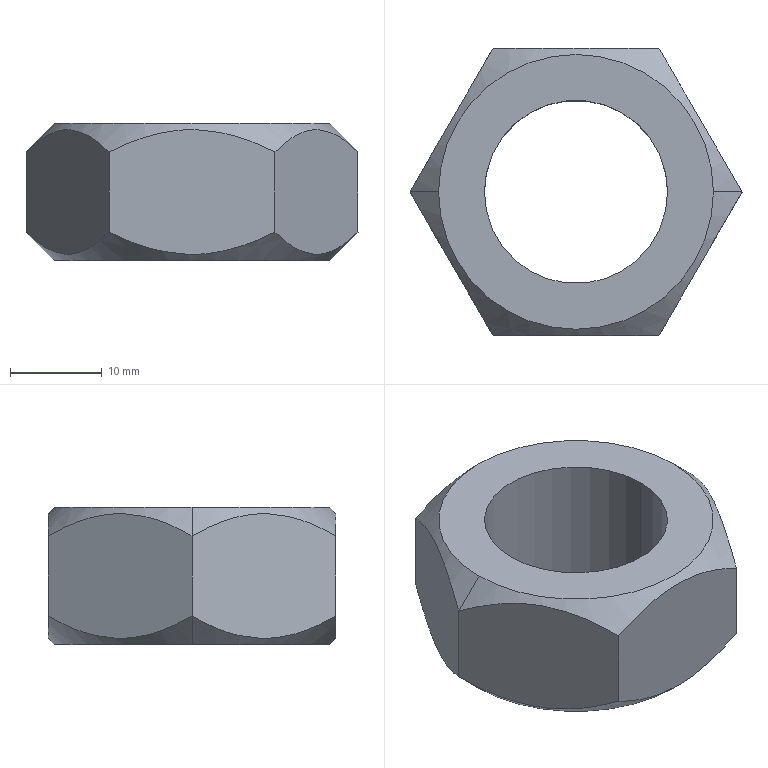Part | Creo | features DATUM PLANE 3, CURVE 2, CHAMFER 1, COORDINATE SYSTEM 1, CUT 1, PROTRUSION 1 | 1 solid | 14 faces | volume 7816 mm3 | plane 8 | cone 4 | cylinder 2 | commonest cylinder face diameters 20 x2